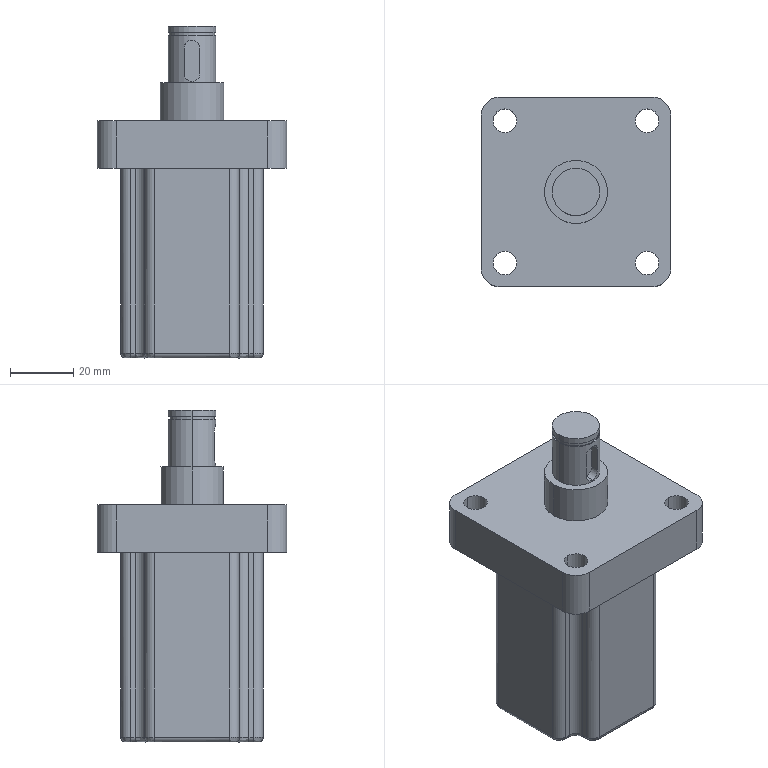Part | SolidWorks | features ICE 5, BaseBody 1 | 1 solid | 89 faces | box 60 x 60 x 105 mm | volume 154768 mm3 | cylinder 49 | plane 28 | spline 12 | commonest cylinder face diameters 3 x12 6 x12 7.5 x8 15 x6 12 x4 5 x3